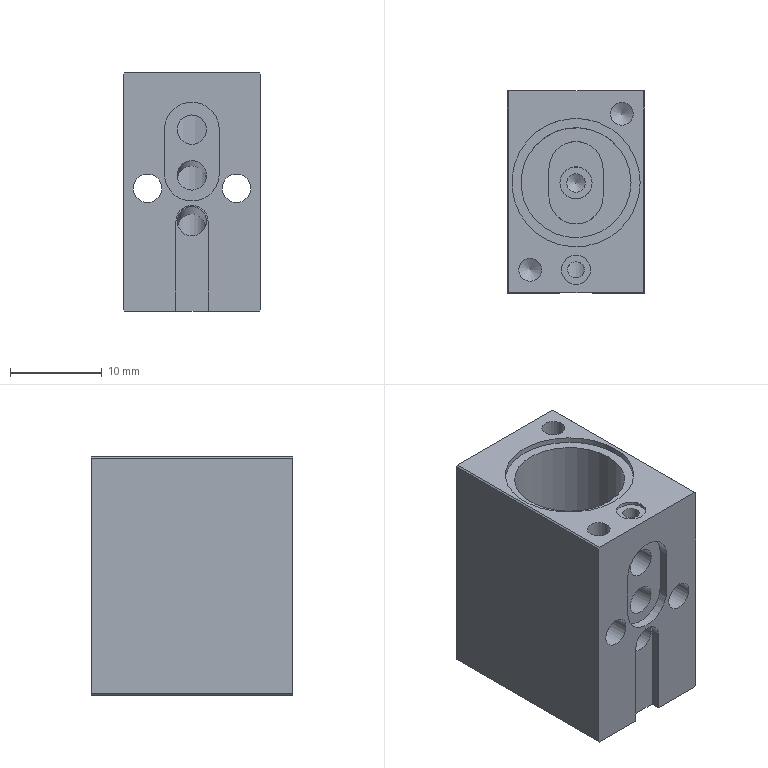Part | 1 solid | 44 faces | box 15 x 22 x 26 mm | volume 6533 mm3 | plane 23 | cylinder 18 | cone 3 | commonest cylinder face diameters 3.2 x4 2.5 x2 3.1 x2 3.5 x2 5.9 x2 6 x2
STEP:
#1=CARTESIAN_POINT('',(-0.01528,-10.,-17.794));
#2=VERTEX_POINT('',#1);
#3=CARTESIAN_POINT('',(-0.01528,-10.,-16.187));
#4=DIRECTION('',(0.,-1.,0.));
#5=DIRECTION('',(0.,0.,-1.));
#6=AXIS2_PLACEMENT_3D('',#3,#4,#5);
#7=ELLIPSE('',#6,1.606,1.6);
#8=EDGE_CURVE('',#2,#2,#7,.T.);
#9=ORIENTED_EDGE('',*,*,#8,.T.);
#10=EDGE_LOOP('',(#9));
#11=FACE_BOUND('',#10,.T.);
#12=CARTESIAN_POINT('',(1.585,0.2576,-17.085));
#13=VERTEX_POINT('',#12);
#14=CARTESIAN_POINT('',(1.488,0.04632,-16.421));
#15=CARTESIAN_POINT('',(1.635,0.3667,-17.087));
#16=CARTESIAN_POINT('',(1.48,0.03243,-17.741));
#17=CARTESIAN_POINT('',(1.041,-0.4993,-18.341));
#18=CARTESIAN_POINT('',(-0.09545,-0.9433,-18.8));
#19=CARTESIAN_POINT('',(-1.156,-0.4116,-18.266));
#20=CARTESIAN_POINT('',(-1.55,0.1565,-17.663));
#21=CARTESIAN_POINT('',(-1.659,0.4306,-16.969));
#22=CARTESIAN_POINT('',(-1.482,0.02854,-16.351));
#23=CARTESIAN_POINT('',(-1.17,-0.3356,-15.874));
#24=CARTESIAN_POINT('',(-0.6683,-0.6615,-15.489));
#25=CARTESIAN_POINT('',(0.02149,-0.7984,-15.334));
#26=CARTESIAN_POINT('',(0.7057,-0.6441,-15.522));
#27=CARTESIAN_POINT('',(1.186,-0.321,-15.926));
#28=CARTESIAN_POINT('',(1.488,0.04632,-16.421));
#29=CARTESIAN_POINT('',(1.635,0.3667,-17.087));
#30=CARTESIAN_POINT('',(1.48,0.03243,-17.741));
#31=B_SPLINE_CURVE_WITH_KNOTS('',3,(#14,#15,#16,#17,#18,#19,#20,#21,#22,#23,#24,#25,#26,#27,#28,#29,#30),.UNSPECIFIED.,.T.,.F.,(1,1,1,1,1,1,1,1,1,1,1,1,1,1,1,1,1,1,1,1,1),(-0.002067,-0.001378,-0.0006891,0.,0.0006891,0.001378,0.002756,0.004134,0.004824,0.005513,0.006202,0.006891,0.00758,0.008269,0.008958,0.009647,0.01034,0.01103,0.01171,0.0124,0.01378),.UNSPECIFIED.);
#32=EDGE_CURVE('',#13,#13,#31,.T.);
#33=ORIENTED_EDGE('',*,*,#32,.T.);
#34=EDGE_LOOP('',(#33));
#35=FACE_BOUND('',#34,.T.);
#36=CARTESIAN_POINT('',(-0.01528,-11.,-16.1));
#37=DIRECTION('',(0.,0.9962,-0.08716));
#38=DIRECTION('',(1.,0.,0.));
#39=AXIS2_PLACEMENT_3D('',#36,#37,#38);
#40=CYLINDRICAL_SURFACE('',#39,1.6);
#41=ADVANCED_FACE('',(#11,#35),#40,.F.);
#42=CARTESIAN_POINT('',(-0.01528,-10.,-12.794));
#43=VERTEX_POINT('',#42);
#44=CARTESIAN_POINT('',(-0.01528,-10.,-11.187));
#45=DIRECTION('',(0.,1.,0.));
#46=DIRECTION('',(0.,0.,-1.));
#47=AXIS2_PLACEMENT_3D('',#44,#45,#46);
#48=ELLIPSE('',#47,1.606,1.6);
#49=EDGE_CURVE('',#43,#43,#48,.T.);
#50=ORIENTED_EDGE('',*,*,#49,.F.);
#51=EDGE_LOOP('',(#50));
#52=FACE_BOUND('',#51,.T.);
#53=CARTESIAN_POINT('',(1.585,-3.038,-11.797));
#54=VERTEX_POINT('',#53);
#55=CARTESIAN_POINT('',(1.252,-3.284,-10.538));
#56=CARTESIAN_POINT('',(1.756,-2.912,-11.798));
#57=CARTESIAN_POINT('',(1.231,-3.297,-13.05));
#58=CARTESIAN_POINT('',(-0.04409,-3.61,-13.528));
#59=CARTESIAN_POINT('',(-1.301,-3.26,-13.012));
#60=CARTESIAN_POINT('',(-1.785,-2.891,-11.745));
#61=CARTESIAN_POINT('',(-1.246,-3.29,-10.505));
#62=CARTESIAN_POINT('',(0.003559,-3.607,-9.965));
#63=CARTESIAN_POINT('',(1.252,-3.284,-10.538));
#64=CARTESIAN_POINT('',(1.756,-2.912,-11.798));
#65=CARTESIAN_POINT('',(1.231,-3.297,-13.05));
#66=B_SPLINE_CURVE_WITH_KNOTS('',3,(#55,#56,#57,#58,#59,#60,#61,#62,#63,#64,#65),.UNSPECIFIED.,.T.,.F.,(1,1,1,1,1,1,1,1,1,1,1,1,1,1,1),(-0.003834,-0.002556,-0.001278,0.,0.001278,0.002556,0.003834,0.005112,0.006391,0.007669,0.008947,0.01022,0.0115,0.01278,0.01406),.UNSPECIFIED.);
#67=EDGE_CURVE('',#54,#54,#66,.T.);
#68=ORIENTED_EDGE('',*,*,#67,.T.);
#69=EDGE_LOOP('',(#68));
#70=FACE_BOUND('',#69,.T.);
#71=CARTESIAN_POINT('',(-0.01528,-11.,-11.1));
#72=DIRECTION('',(0.,0.9962,-0.08716));
#73=DIRECTION('',(1.,0.,0.));
#74=AXIS2_PLACEMENT_3D('',#71,#72,#73);
#75=CYLINDRICAL_SURFACE('',#74,1.6);
#76=ADVANCED_FACE('',(#52,#70),#75,.F.);
#77=CARTESIAN_POINT('',(2.985,-11.,-11.));
#78=VERTEX_POINT('',#77);
#79=CARTESIAN_POINT('',(-3.015,-11.,-11.));
#80=VERTEX_POINT('',#79);
#81=CARTESIAN_POINT('',(-0.01528,-11.,-11.));
#82=DIRECTION('',(0.,1.,0.));
#83=DIRECTION('',(0.,0.,1.));
#84=AXIS2_PLACEMENT_3D('',#81,#82,#83);
#85=CIRCLE('',#84,3.);
#86=EDGE_CURVE('',#78,#80,#85,.T.);
#87=ORIENTED_EDGE('',*,*,#86,.T.);
#88=CARTESIAN_POINT('',(-3.015,-11.,-6.2));
#89=VERTEX_POINT('',#88);
#90=CARTESIAN_POINT('',(-3.015,-11.,-11.));
#91=DIRECTION('',(0.,0.,1.));
#92=VECTOR('',#91,1000.);
#93=LINE('',#90,#92);
#94=EDGE_CURVE('',#80,#89,#93,.T.);
#95=ORIENTED_EDGE('',*,*,#94,.T.);
#96=CARTESIAN_POINT('',(2.985,-11.,-6.2));
#97=VERTEX_POINT('',#96);
#98=CARTESIAN_POINT('',(-0.01528,-11.,-6.2));
#99=DIRECTION('',(0.,1.,0.));
#100=DIRECTION('',(0.,0.,1.));
#101=AXIS2_PLACEMENT_3D('',#98,#99,#100);
#102=CIRCLE('',#101,3.);
#103=EDGE_CURVE('',#89,#97,#102,.T.);
#104=ORIENTED_EDGE('',*,*,#103,.T.);
#105=CARTESIAN_POINT('',(2.985,-11.,-6.2));
#106=DIRECTION('',(0.,0.,-1.));
#107=VECTOR('',#106,1000.);
#108=LINE('',#105,#107);
#109=EDGE_CURVE('',#97,#78,#108,.T.);
#110=ORIENTED_EDGE('',*,*,#109,.T.);
#111=EDGE_LOOP('',(#87,#95,#104,#110));
#112=FACE_BOUND('',#111,.T.);
#113=CARTESIAN_POINT('',(4.85,-11.,-11.05));
#114=VERTEX_POINT('',#113);
#115=CARTESIAN_POINT('',(4.85,-11.,-12.6));
#116=DIRECTION('',(0.,1.,0.));
#117=DIRECTION('',(0.,0.,1.));
#118=AXIS2_PLACEMENT_3D('',#115,#116,#117);
#119=CIRCLE('',#118,1.55);
#120=EDGE_CURVE('',#114,#114,#119,.T.);
#121=ORIENTED_EDGE('',*,*,#120,.T.);
#122=EDGE_LOOP('',(#121));
#123=FACE_BOUND('',#122,.T.);
#124=CARTESIAN_POINT('',(-4.85,-11.,-11.05));
#125=VERTEX_POINT('',#124);
#126=CARTESIAN_POINT('',(-4.85,-11.,-12.6));
#127=DIRECTION('',(0.,1.,0.));
#128=DIRECTION('',(0.,0.,1.));
#129=AXIS2_PLACEMENT_3D('',#126,#127,#128);
#130=CIRCLE('',#129,1.55);
#131=EDGE_CURVE('',#125,#125,#130,.T.);
#132=ORIENTED_EDGE('',*,*,#131,.T.);
#133=EDGE_LOOP('',(#132));
#134=FACE_BOUND('',#133,.T.);
#135=CARTESIAN_POINT('',(-7.5,-11.,-25.85));
#136=VERTEX_POINT('',#135);
#137=CARTESIAN_POINT('',(-7.5,-11.,-0.15));
#138=VERTEX_POINT('',#137);
#139=CARTESIAN_POINT('',(-7.5,-11.,-26.));
#140=DIRECTION('',(0.,0.,1.));
#141=VECTOR('',#140,1000.);
#142=LINE('',#139,#141);
#143=EDGE_CURVE('',#136,#138,#142,.T.);
#144=ORIENTED_EDGE('',*,*,#143,.F.);
#145=CARTESIAN_POINT('',(-7.35,-11.,-26.));
#146=VERTEX_POINT('',#145);
#147=CARTESIAN_POINT('',(-7.35,-11.,-26.));
#148=DIRECTION('',(0.7071,0.,-0.7071));
#149=VECTOR('',#148,1000.);
#150=LINE('',#147,#149);
#151=EDGE_CURVE('',#136,#146,#150,.T.);
#152=ORIENTED_EDGE('',*,*,#151,.T.);
#153=CARTESIAN_POINT('',(-1.75,-11.,-26.));
#154=VERTEX_POINT('',#153);
#155=CARTESIAN_POINT('',(7.5,-11.,-26.));
#156=DIRECTION('',(-1.,0.,0.));
#157=VECTOR('',#156,1000.);
#158=LINE('',#155,#157);
#159=EDGE_CURVE('',#154,#146,#158,.T.);
#160=ORIENTED_EDGE('',*,*,#159,.F.);
#161=CARTESIAN_POINT('',(-1.75,-11.,-16.2));
#162=VERTEX_POINT('',#161);
#163=CARTESIAN_POINT('',(-1.75,-11.,-16.2));
#164=DIRECTION('',(0.,0.,-1.));
#165=VECTOR('',#164,1000.);
#166=LINE('',#163,#165);
#167=EDGE_CURVE('',#162,#154,#166,.T.);
#168=ORIENTED_EDGE('',*,*,#167,.F.);
#169=CARTESIAN_POINT('',(1.75,-11.,-16.2));
#170=VERTEX_POINT('',#169);
#171=CARTESIAN_POINT('',(0.,-11.,-16.2));
#172=DIRECTION('',(0.,-1.,0.));
#173=DIRECTION('',(0.,0.,1.));
#174=AXIS2_PLACEMENT_3D('',#171,#172,#173);
#175=CIRCLE('',#174,1.75);
#176=EDGE_CURVE('',#170,#162,#175,.T.);
#177=ORIENTED_EDGE('',*,*,#176,.F.);
#178=CARTESIAN_POINT('',(1.75,-11.,-26.));
#179=VERTEX_POINT('',#178);
#180=CARTESIAN_POINT('',(1.75,-11.,-26.));
#181=DIRECTION('',(0.,0.,1.));
#182=VECTOR('',#181,1000.);
#183=LINE('',#180,#182);
#184=EDGE_CURVE('',#179,#170,#183,.T.);
#185=ORIENTED_EDGE('',*,*,#184,.F.);
#186=CARTESIAN_POINT('',(7.35,-11.,-26.));
#187=VERTEX_POINT('',#186);
#188=CARTESIAN_POINT('',(7.5,-11.,-26.));
#189=DIRECTION('',(-1.,0.,0.));
#190=VECTOR('',#189,1000.);
#191=LINE('',#188,#190);
#192=EDGE_CURVE('',#187,#179,#191,.T.);
#193=ORIENTED_EDGE('',*,*,#192,.F.);
#194=CARTESIAN_POINT('',(7.5,-11.,-25.85));
#195=VERTEX_POINT('',#194);
#196=CARTESIAN_POINT('',(7.35,-11.,-26.));
#197=DIRECTION('',(0.7071,0.,0.7071));
#198=VECTOR('',#197,1000.);
#199=LINE('',#196,#198);
#200=EDGE_CURVE('',#187,#195,#199,.T.);
#201=ORIENTED_EDGE('',*,*,#200,.T.);
#202=CARTESIAN_POINT('',(7.5,-11.,-0.15));
#203=VERTEX_POINT('',#202);
#204=CARTESIAN_POINT('',(7.5,-11.,-26.));
#205=DIRECTION('',(0.,0.,1.));
#206=VECTOR('',#205,1000.);
#207=LINE('',#204,#206);
#208=EDGE_CURVE('',#195,#203,#207,.T.);
#209=ORIENTED_EDGE('',*,*,#208,.T.);
#210=CARTESIAN_POINT('',(7.35,-11.,0.));
#211=VERTEX_POINT('',#210);
#212=CARTESIAN_POINT('',(7.5,-11.,-0.15));
#213=DIRECTION('',(0.7071,0.,-0.7071));
#214=VECTOR('',#213,1000.);
#215=LINE('',#212,#214);
#216=EDGE_CURVE('',#203,#211,#215,.F.);
#217=ORIENTED_EDGE('',*,*,#216,.T.);
#218=CARTESIAN_POINT('',(-7.35,-11.,0.));
#219=VERTEX_POINT('',#218);
#220=CARTESIAN_POINT('',(7.5,-11.,0.));
#221=DIRECTION('',(-1.,0.,0.));
#222=VECTOR('',#221,1000.);
#223=LINE('',#220,#222);
#224=EDGE_CURVE('',#211,#219,#223,.T.);
#225=ORIENTED_EDGE('',*,*,#224,.T.);
#226=CARTESIAN_POINT('',(-7.5,-11.,-0.15));
#227=DIRECTION('',(0.7071,0.,0.7071));
#228=VECTOR('',#227,1000.);
#229=LINE('',#226,#228);
#230=EDGE_CURVE('',#219,#138,#229,.F.);
#231=ORIENTED_EDGE('',*,*,#230,.T.);
#232=EDGE_LOOP('',(#144,#152,#160,#168,#177,#185,#193,#201,#209,#217,#225,#231));
#233=FACE_BOUND('',#232,.T.);
#234=CARTESIAN_POINT('',(7.5,-11.,-26.));
#235=DIRECTION('',(0.,1.,0.));
#236=DIRECTION('',(0.,0.,1.));
#237=AXIS2_PLACEMENT_3D('',#234,#235,#236);
#238=PLANE('',#237);
#239=ADVANCED_FACE('',(#112,#123,#134,#233),#238,.F.);
#240=ORIENTED_EDGE('',*,*,#159,.T.);
#241=CARTESIAN_POINT('',(-7.35,11.,-26.));
#242=VERTEX_POINT('',#241);
#243=CARTESIAN_POINT('',(-7.35,11.,-26.));
#244=DIRECTION('',(0.,1.,0.));
#245=VECTOR('',#244,1000.);
#246=LINE('',#243,#245);
#247=EDGE_CURVE('',#146,#242,#246,.T.);
#248=ORIENTED_EDGE('',*,*,#247,.T.);
#249=CARTESIAN_POINT('',(7.35,11.,-26.));
#250=VERTEX_POINT('',#249);
#251=CARTESIAN_POINT('',(-7.5,11.,-26.));
#252=DIRECTION('',(1.,0.,0.));
#253=VECTOR('',#252,1000.);
#254=LINE('',#251,#253);
#255=EDGE_CURVE('',#242,#250,#254,.T.);
#256=ORIENTED_EDGE('',*,*,#255,.T.);
#257=CARTESIAN_POINT('',(7.35,-11.,-26.));
#258=DIRECTION('',(0.,-1.,0.));
#259=VECTOR('',#258,1000.);
#260=LINE('',#257,#259);
#261=EDGE_CURVE('',#250,#187,#260,.T.);
#262=ORIENTED_EDGE('',*,*,#261,.T.);
#263=ORIENTED_EDGE('',*,*,#192,.T.);
#264=CARTESIAN_POINT('',(1.75,-10.,-26.));
#265=VERTEX_POINT('',#264);
#266=CARTESIAN_POINT('',(1.75,-10.,-26.));
#267=DIRECTION('',(0.,-1.,0.));
#268=VECTOR('',#267,1000.);
#269=LINE('',#266,#268);
#270=EDGE_CURVE('',#265,#179,#269,.T.);
#271=ORIENTED_EDGE('',*,*,#270,.F.);
#272=CARTESIAN_POINT('',(-1.75,-10.,-26.));
#273=VERTEX_POINT('',#272);
#274=CARTESIAN_POINT('',(-1.75,-10.,-26.));
#275=DIRECTION('',(1.,0.,0.));
#276=VECTOR('',#275,1000.);
#277=LINE('',#274,#276);
#278=EDGE_CURVE('',#273,#265,#277,.T.);
#279=ORIENTED_EDGE('',*,*,#278,.F.);
#280=CARTESIAN_POINT('',(-1.75,-10.,-26.));
#281=DIRECTION('',(0.,-1.,0.));
#282=VECTOR('',#281,1000.);
#283=LINE('',#280,#282);
#284=EDGE_CURVE('',#273,#154,#283,.T.);
#285=ORIENTED_EDGE('',*,*,#284,.T.);
#286=EDGE_LOOP('',(#240,#248,#256,#262,#263,#271,#279,#285));
#287=FACE_BOUND('',#286,.T.);
#288=CARTESIAN_POINT('',(0.,0.,-26.));
#289=DIRECTION('',(0.,0.,-1.));
#290=DIRECTION('',(-1.,0.,0.));
#291=AXIS2_PLACEMENT_3D('',#288,#289,#290);
#292=PLANE('',#291);
#293=ADVANCED_FACE('',(#287),#292,.T.);
#294=ORIENTED_EDGE('',*,*,#131,.F.);
#295=EDGE_LOOP('',(#294));
#296=FACE_BOUND('',#295,.T.);
#297=CARTESIAN_POINT('',(-4.85,11.,-14.15));
#298=VERTEX_POINT('',#297);
#299=CARTESIAN_POINT('',(-4.85,11.,-12.6));
#300=DIRECTION('',(0.,-1.,0.));
#301=DIRECTION('',(0.,0.,-1.));
#302=AXIS2_PLACEMENT_3D('',#299,#300,#301);
#303=CIRCLE('',#302,1.55);
#304=EDGE_CURVE('',#298,#298,#303,.F.);
#305=ORIENTED_EDGE('',*,*,#304,.T.);
#306=EDGE_LOOP('',(#305));
#307=FACE_BOUND('',#306,.T.);
#308=CARTESIAN_POINT('',(-4.85,-11.,-12.6));
#309=DIRECTION('',(0.,1.,0.));
#310=DIRECTION('',(1.,0.,0.));
#311=AXIS2_PLACEMENT_3D('',#308,#309,#310);
#312=CYLINDRICAL_SURFACE('',#311,1.55);
#313=ADVANCED_FACE('',(#296,#307),#312,.F.);
#314=CARTESIAN_POINT('',(-7.5,11.,-25.85));
#315=VERTEX_POINT('',#314);
#316=CARTESIAN_POINT('',(-7.5,11.,-0.15));
#317=VERTEX_POINT('',#316);
#318=CARTESIAN_POINT('',(-7.5,11.,-26.));
#319=DIRECTION('',(0.,0.,1.));
#320=VECTOR('',#319,1000.);
#321=LINE('',#318,#320);
#322=EDGE_CURVE('',#315,#317,#321,.T.);
#323=ORIENTED_EDGE('',*,*,#322,.F.);
#324=CARTESIAN_POINT('',(-7.5,-11.,-25.85));
#325=DIRECTION('',(0.,-1.,0.));
#326=VECTOR('',#325,1000.);
#327=LINE('',#324,#326);
#328=EDGE_CURVE('',#315,#136,#327,.T.);
#329=ORIENTED_EDGE('',*,*,#328,.T.);
#330=ORIENTED_EDGE('',*,*,#143,.T.);
#331=CARTESIAN_POINT('',(-7.5,-11.,-0.15));
#332=DIRECTION('',(0.,1.,0.));
#333=VECTOR('',#332,1000.);
#334=LINE('',#331,#333);
#335=EDGE_CURVE('',#138,#317,#334,.T.);
#336=ORIENTED_EDGE('',*,*,#335,.T.);
#337=EDGE_LOOP('',(#323,#329,#330,#336));
#338=FACE_BOUND('',#337,.T.);
#339=CARTESIAN_POINT('',(-7.5,-11.,-26.));
#340=DIRECTION('',(1.,0.,0.));
#341=DIRECTION('',(0.,0.,-1.));
#342=AXIS2_PLACEMENT_3D('',#339,#340,#341);
#343=PLANE('',#342);
#344=ADVANCED_FACE('',(#338),#343,.F.);
#345=ORIENTED_EDGE('',*,*,#304,.F.);
#346=EDGE_LOOP('',(#345));
#347=FACE_BOUND('',#346,.T.);
#348=CARTESIAN_POINT('',(4.85,11.,-14.15));
#349=VERTEX_POINT('',#348);
#350=CARTESIAN_POINT('',(4.85,11.,-12.6));
#351=DIRECTION('',(0.,-1.,0.));
#352=DIRECTION('',(0.,0.,-1.));
#353=AXIS2_PLACEMENT_3D('',#350,#351,#352);
#354=CIRCLE('',#353,1.55);
#355=EDGE_CURVE('',#349,#349,#354,.T.);
#356=ORIENTED_EDGE('',*,*,#355,.T.);
#357=EDGE_LOOP('',(#356));
#358=FACE_BOUND('',#357,.T.);
#359=ORIENTED_EDGE('',*,*,#255,.F.);
#360=CARTESIAN_POINT('',(-7.35,11.,-26.));
#361=DIRECTION('',(-0.7071,0.,0.7071));
#362=VECTOR('',#361,1000.);
#363=LINE('',#360,#362);
#364=EDGE_CURVE('',#242,#315,#363,.T.);
#365=ORIENTED_EDGE('',*,*,#364,.T.);
#366=ORIENTED_EDGE('',*,*,#322,.T.);
#367=CARTESIAN_POINT('',(-7.35,11.,0.));
#368=VERTEX_POINT('',#367);
#369=CARTESIAN_POINT('',(-7.5,11.,-0.15));
#370=DIRECTION('',(-0.7071,0.,-0.7071));
#371=VECTOR('',#370,1000.);
#372=LINE('',#369,#371);
#373=EDGE_CURVE('',#317,#368,#372,.F.);
#374=ORIENTED_EDGE('',*,*,#373,.T.);
#375=CARTESIAN_POINT('',(7.35,11.,0.));
#376=VERTEX_POINT('',#375);
#377=CARTESIAN_POINT('',(-7.5,11.,0.));
#378=DIRECTION('',(1.,0.,0.));
#379=VECTOR('',#378,1000.);
#380=LINE('',#377,#379);
#381=EDGE_CURVE('',#368,#376,#380,.T.);
#382=ORIENTED_EDGE('',*,*,#381,.T.);
#383=CARTESIAN_POINT('',(7.5,11.,-0.15));
#384=VERTEX_POINT('',#383);
#385=CARTESIAN_POINT('',(7.5,11.,-0.15));
#386=DIRECTION('',(-0.7071,0.,0.7071));
#387=VECTOR('',#386,1000.);
#388=LINE('',#385,#387);
#389=EDGE_CURVE('',#376,#384,#388,.F.);
#390=ORIENTED_EDGE('',*,*,#389,.T.);
#391=CARTESIAN_POINT('',(7.5,11.,-25.85));
#392=VERTEX_POINT('',#391);
#393=CARTESIAN_POINT('',(7.5,11.,-26.));
#394=DIRECTION('',(0.,0.,1.));
#395=VECTOR('',#394,1000.);
#396=LINE('',#393,#395);
#397=EDGE_CURVE('',#392,#384,#396,.T.);
#398=ORIENTED_EDGE('',*,*,#397,.F.);
#399=CARTESIAN_POINT('',(7.35,11.,-26.));
#400=DIRECTION('',(-0.7071,0.,-0.7071));
#401=VECTOR('',#400,1000.);
#402=LINE('',#399,#401);
#403=EDGE_CURVE('',#392,#250,#402,.T.);
#404=ORIENTED_EDGE('',*,*,#403,.T.);
#405=EDGE_LOOP('',(#359,#365,#366,#374,#382,#390,#398,#404));
#406=FACE_BOUND('',#405,.T.);
#407=CARTESIAN_POINT('',(-7.5,11.,-26.));
#408=DIRECTION('',(0.,-1.,0.));
#409=DIRECTION('',(0.,0.,-1.));
#410=AXIS2_PLACEMENT_3D('',#407,#408,#409);
#411=PLANE('',#410);
#412=ADVANCED_FACE('',(#347,#358,#406),#411,.F.);
#413=ORIENTED_EDGE('',*,*,#208,.F.);
#414=CARTESIAN_POINT('',(7.5,11.,-25.85));
#415=DIRECTION('',(0.,1.,0.));
#416=VECTOR('',#415,1000.);
#417=LINE('',#414,#416);
#418=EDGE_CURVE('',#195,#392,#417,.T.);
#419=ORIENTED_EDGE('',*,*,#418,.T.);
#420=ORIENTED_EDGE('',*,*,#397,.T.);
#421=CARTESIAN_POINT('',(7.5,11.,-0.15));
#422=DIRECTION('',(0.,-1.,0.));
#423=VECTOR('',#422,1000.);
#424=LINE('',#421,#423);
#425=EDGE_CURVE('',#384,#203,#424,.T.);
#426=ORIENTED_EDGE('',*,*,#425,.T.);
#427=EDGE_LOOP('',(#413,#419,#420,#426));
#428=FACE_BOUND('',#427,.T.);
#429=CARTESIAN_POINT('',(7.5,11.,-26.));
#430=DIRECTION('',(-1.,0.,0.));
#431=DIRECTION('',(0.,0.,1.));
#432=AXIS2_PLACEMENT_3D('',#429,#430,#431);
#433=PLANE('',#432);
#434=ADVANCED_FACE('',(#428),#433,.F.);
#435=CARTESIAN_POINT('',(1.6,-8.5,0.));
#436=VERTEX_POINT('',#435);
#437=CARTESIAN_POINT('',(0.,-8.5,0.));
#438=DIRECTION('',(0.,0.,1.));
#439=DIRECTION('',(1.,0.,0.));
#440=AXIS2_PLACEMENT_3D('',#437,#438,#439);
#441=CIRCLE('',#440,1.6);
#442=EDGE_CURVE('',#436,#436,#441,.T.);
#443=ORIENTED_EDGE('',*,*,#442,.F.);
#444=EDGE_LOOP('',(#443));
#445=FACE_BOUND('',#444,.T.);
#446=CARTESIAN_POINT('',(-6.25,-8.5,0.));
#447=VERTEX_POINT('',#446);
#448=CARTESIAN_POINT('',(-5.,-8.5,0.));
#449=DIRECTION('',(0.,0.,-1.));
#450=DIRECTION('',(-1.,0.,0.));
#451=AXIS2_PLACEMENT_3D('',#448,#449,#450);
#452=CIRCLE('',#451,1.25);
#453=EDGE_CURVE('',#447,#447,#452,.T.);
#454=ORIENTED_EDGE('',*,*,#453,.T.);
#455=EDGE_LOOP('',(#454));
#456=FACE_BOUND('',#455,.T.);
#457=CARTESIAN_POINT('',(3.75,8.5,0.));
#458=VERTEX_POINT('',#457);
#459=CARTESIAN_POINT('',(5.,8.5,0.));
#460=DIRECTION('',(0.,0.,-1.));
#461=DIRECTION('',(-1.,0.,0.));
#462=AXIS2_PLACEMENT_3D('',#459,#460,#461);
#463=CIRCLE('',#462,1.25);
#464=EDGE_CURVE('',#458,#458,#463,.T.);
#465=ORIENTED_EDGE('',*,*,#464,.T.);
#466=EDGE_LOOP('',(#465));
#467=FACE_BOUND('',#466,.T.);
#468=CARTESIAN_POINT('',(7.,1.,0.));
#469=VERTEX_POINT('',#468);
#470=CARTESIAN_POINT('',(0.,1.,0.));
#471=DIRECTION('',(0.,0.,1.));
#472=DIRECTION('',(1.,0.,0.));
#473=AXIS2_PLACEMENT_3D('',#470,#471,#472);
#474=CIRCLE('',#473,7.);
#475=EDGE_CURVE('',#469,#469,#474,.T.);
#476=ORIENTED_EDGE('',*,*,#475,.F.);
#477=EDGE_LOOP('',(#476));
#478=FACE_BOUND('',#477,.T.);
#479=ORIENTED_EDGE('',*,*,#224,.F.);
#480=CARTESIAN_POINT('',(7.35,0.,0.));
#481=DIRECTION('',(0.,1.,0.));
#482=VECTOR('',#481,1000.);
#483=LINE('',#480,#482);
#484=EDGE_CURVE('',#211,#376,#483,.T.);
#485=ORIENTED_EDGE('',*,*,#484,.T.);
#486=ORIENTED_EDGE('',*,*,#381,.F.);
#487=CARTESIAN_POINT('',(-7.35,0.,0.));
#488=DIRECTION('',(0.,-1.,0.));
#489=VECTOR('',#488,1000.);
#490=LINE('',#487,#489);
#491=EDGE_CURVE('',#368,#219,#490,.T.);
#492=ORIENTED_EDGE('',*,*,#491,.T.);
#493=EDGE_LOOP('',(#479,#485,#486,#492));
#494=FACE_BOUND('',#493,.T.);
#495=CARTESIAN_POINT('',(0.,0.,0.));
#496=DIRECTION('',(0.,0.,-1.));
#497=DIRECTION('',(-1.,0.,0.));
#498=AXIS2_PLACEMENT_3D('',#495,#496,#497);
#499=PLANE('',#498);
#500=ADVANCED_FACE('',(#445,#456,#467,#478,#494),#499,.F.);
#501=CARTESIAN_POINT('',(7.,1.,-0.6));
#502=VERTEX_POINT('',#501);
#503=CARTESIAN_POINT('',(0.,1.,-0.6));
#504=DIRECTION('',(0.,0.,1.));
#505=DIRECTION('',(1.,0.,0.));
#506=AXIS2_PLACEMENT_3D('',#503,#504,#505);
#507=CIRCLE('',#506,7.);
#508=EDGE_CURVE('',#502,#502,#507,.F.);
#509=ORIENTED_EDGE('',*,*,#508,.T.);
#510=EDGE_LOOP('',(#509));
#511=FACE_BOUND('',#510,.T.);
#512=ORIENTED_EDGE('',*,*,#475,.T.);
#513=EDGE_LOOP('',(#512));
#514=FACE_BOUND('',#513,.T.);
#515=CARTESIAN_POINT('',(0.,1.,-0.6));
#516=DIRECTION('',(0.,0.,1.));
#517=DIRECTION('',(1.,0.,0.));
#518=AXIS2_PLACEMENT_3D('',#515,#516,#517);
#519=CYLINDRICAL_SURFACE('',#518,7.);
#520=ADVANCED_FACE('',(#511,#514),#519,.F.);
#521=CARTESIAN_POINT('',(6.,1.,-0.6));
#522=VERTEX_POINT('',#521);
#523=CARTESIAN_POINT('',(0.,1.,-0.6));
#524=DIRECTION('',(0.,0.,1.));
#525=DIRECTION('',(1.,0.,0.));
#526=AXIS2_PLACEMENT_3D('',#523,#524,#525);
#527=CIRCLE('',#526,6.);
#528=EDGE_CURVE('',#522,#522,#527,.T.);
#529=ORIENTED_EDGE('',*,*,#528,.F.);
#530=EDGE_LOOP('',(#529));
#531=FACE_BOUND('',#530,.T.);
#532=ORIENTED_EDGE('',*,*,#508,.F.);
#533=EDGE_LOOP('',(#532));
#534=FACE_BOUND('',#533,.T.);
#535=CARTESIAN_POINT('',(0.,1.,-0.6));
#536=DIRECTION('',(0.,0.,1.));
#537=DIRECTION('',(1.,0.,0.));
#538=AXIS2_PLACEMENT_3D('',#535,#536,#537);
#539=PLANE('',#538);
#540=ADVANCED_FACE('',(#531,#534),#539,.T.);
#541=CARTESIAN_POINT('',(-0.01528,-5.,-4.6));
#542=VERTEX_POINT('',#541);
#543=CARTESIAN_POINT('',(1.24,-4.896,-4.947));
#544=CARTESIAN_POINT('',(-0.01563,-5.053,-4.426));
#545=CARTESIAN_POINT('',(-1.269,-4.89,-4.947));
#546=CARTESIAN_POINT('',(-1.788,-4.723,-6.198));
#547=CARTESIAN_POINT('',(-1.269,-4.89,-7.454));
#548=CARTESIAN_POINT('',(-0.01711,-5.053,-7.973));
#549=CARTESIAN_POINT('',(1.237,-4.897,-7.455));
#550=CARTESIAN_POINT('',(1.758,-4.732,-6.201));
#551=CARTESIAN_POINT('',(1.24,-4.896,-4.947));
#552=CARTESIAN_POINT('',(-0.01563,-5.053,-4.426));
#553=CARTESIAN_POINT('',(-1.269,-4.89,-4.947));
#554=B_SPLINE_CURVE_WITH_KNOTS('',3,(#543,#544,#545,#546,#547,#548,#549,#550,#551,#552,#553),.UNSPECIFIED.,.T.,.F.,(1,1,1,1,1,1,1,1,1,1,1,1,1,1,1),(-0.003768,-0.002512,-0.001256,0.,0.001256,0.002512,0.003768,0.005024,0.006281,0.007537,0.008793,0.01005,0.01131,0.01256,0.01382),.UNSPECIFIED.);
#555=EDGE_CURVE('',#542,#542,#554,.T.);
#556=ORIENTED_EDGE('',*,*,#555,.T.);
#557=EDGE_LOOP('',(#556));
#558=FACE_BOUND('',#557,.T.);
#559=ORIENTED_EDGE('',*,*,#528,.T.);
#560=EDGE_LOOP('',(#559));
#561=FACE_BOUND('',#560,.T.);
#562=CARTESIAN_POINT('',(6.,1.,-9.2));
#563=VERTEX_POINT('',#562);
#564=CARTESIAN_POINT('',(0.,1.,-9.2));
#565=DIRECTION('',(0.,0.,1.));
#566=DIRECTION('',(1.,0.,0.));
#567=AXIS2_PLACEMENT_3D('',#564,#565,#566);
#568=CIRCLE('',#567,6.);
#569=EDGE_CURVE('',#563,#563,#568,.F.);
#570=ORIENTED_EDGE('',*,*,#569,.T.);
#571=EDGE_LOOP('',(#570));
#572=FACE_BOUND('',#571,.T.);
#573=CARTESIAN_POINT('',(0.,1.,-9.2));
#574=DIRECTION('',(0.,0.,1.));
#575=DIRECTION('',(1.,0.,0.));
#576=AXIS2_PLACEMENT_3D('',#573,#574,#575);
#577=CYLINDRICAL_SURFACE('',#576,6.);
#578=ADVANCED_FACE('',(#558,#561,#572),#577,.F.);
#579=CARTESIAN_POINT('',(2.95,2.55,-9.2));
#580=VERTEX_POINT('',#579);
#581=CARTESIAN_POINT('',(-2.95,2.55,-9.2));
#582=VERTEX_POINT('',#581);
#583=CARTESIAN_POINT('',(0.,2.55,-9.2));
#584=DIRECTION('',(0.,0.,1.));
#585=DIRECTION('',(1.,0.,0.));
#586=AXIS2_PLACEMENT_3D('',#583,#584,#585);
#587=CIRCLE('',#586,2.95);
#588=EDGE_CURVE('',#580,#582,#587,.T.);
#589=ORIENTED_EDGE('',*,*,#588,.F.);
#590=CARTESIAN_POINT('',(2.95,-0.55,-9.2));
#591=VERTEX_POINT('',#590);
#592=CARTESIAN_POINT('',(2.95,1.,-9.2));
#593=DIRECTION('',(0.,1.,0.));
#594=VECTOR('',#593,1000.);
#595=LINE('',#592,#594);
#596=EDGE_CURVE('',#591,#580,#595,.T.);
#597=ORIENTED_EDGE('',*,*,#596,.F.);
#598=CARTESIAN_POINT('',(-2.95,-0.55,-9.2));
#599=VERTEX_POINT('',#598);
#600=CARTESIAN_POINT('',(0.,-0.55,-9.2));
#601=DIRECTION('',(0.,0.,1.));
#602=DIRECTION('',(1.,0.,0.));
#603=AXIS2_PLACEMENT_3D('',#600,#601,#602);
#604=CIRCLE('',#603,2.95);
#605=EDGE_CURVE('',#599,#591,#604,.T.);
#606=ORIENTED_EDGE('',*,*,#605,.F.);
#607=CARTESIAN_POINT('',(-2.95,1.,-9.2));
#608=DIRECTION('',(0.,-1.,0.));
#609=VECTOR('',#608,1000.);
#610=LINE('',#607,#609);
#611=EDGE_CURVE('',#582,#599,#610,.T.);
#612=ORIENTED_EDGE('',*,*,#611,.F.);
#613=EDGE_LOOP('',(#589,#597,#606,#612));
#614=FACE_BOUND('',#613,.T.);
#615=ORIENTED_EDGE('',*,*,#569,.F.);
#616=EDGE_LOOP('',(#615));
#617=FACE_BOUND('',#616,.T.);
#618=CARTESIAN_POINT('',(0.,1.,-9.2));
#619=DIRECTION('',(0.,0.,1.));
#620=DIRECTION('',(1.,0.,0.));
#621=AXIS2_PLACEMENT_3D('',#618,#619,#620);
#622=PLANE('',#621);
#623=ADVANCED_FACE('',(#614,#617),#622,.T.);
#624=ORIENTED_EDGE('',*,*,#588,.T.);
#625=CARTESIAN_POINT('',(-2.95,2.55,-13.7));
#626=VERTEX_POINT('',#625);
#627=CARTESIAN_POINT('',(-2.95,2.55,-13.8));
#628=DIRECTION('',(0.,0.,1.));
#629=VECTOR('',#628,1000.);
#630=LINE('',#627,#629);
#631=EDGE_CURVE('',#582,#626,#630,.F.);
#632=ORIENTED_EDGE('',*,*,#631,.T.);
#633=CARTESIAN_POINT('',(2.95,2.55,-13.7));
#634=VERTEX_POINT('',#633);
#635=CARTESIAN_POINT('',(0.,2.55,-13.7));
#636=DIRECTION('',(0.,0.,1.));
#637=DIRECTION('',(1.,0.,0.));
#638=AXIS2_PLACEMENT_3D('',#635,#636,#637);
#639=CIRCLE('',#638,2.95);
#640=EDGE_CURVE('',#626,#634,#639,.F.);
#641=ORIENTED_EDGE('',*,*,#640,.T.);
#642=CARTESIAN_POINT('',(2.95,2.55,-13.8));
#643=DIRECTION('',(0.,0.,1.));
#644=VECTOR('',#643,1000.);
#645=LINE('',#642,#644);
#646=EDGE_CURVE('',#580,#634,#645,.F.);
#647=ORIENTED_EDGE('',*,*,#646,.F.);
#648=EDGE_LOOP('',(#624,#632,#641,#647));
#649=FACE_BOUND('',#648,.T.);
#650=CARTESIAN_POINT('',(0.,2.55,-13.8));
#651=DIRECTION('',(0.,0.,1.));
#652=DIRECTION('',(1.,0.,0.));
#653=AXIS2_PLACEMENT_3D('',#650,#651,#652);
#654=CYLINDRICAL_SURFACE('',#653,2.95);
#655=ADVANCED_FACE('',(#649),#654,.F.);
#656=ORIENTED_EDGE('',*,*,#611,.T.);
#657=CARTESIAN_POINT('',(-2.95,-0.55,-13.7));
#658=VERTEX_POINT('',#657);
#659=CARTESIAN_POINT('',(-2.95,-0.55,-13.8));
#660=DIRECTION('',(0.,0.,1.));
#661=VECTOR('',#660,1000.);
#662=LINE('',#659,#661);
#663=EDGE_CURVE('',#599,#658,#662,.F.);
#664=ORIENTED_EDGE('',*,*,#663,.T.);
#665=CARTESIAN_POINT('',(-2.95,2.4,-13.7));
#666=DIRECTION('',(0.,1.,0.));
#667=VECTOR('',#666,1000.);
#668=LINE('',#665,#667);
#669=EDGE_CURVE('',#658,#626,#668,.T.);
#670=ORIENTED_EDGE('',*,*,#669,.T.);
#671=ORIENTED_EDGE('',*,*,#631,.F.);
#672=EDGE_LOOP('',(#656,#664,#670,#671));
#673=FACE_BOUND('',#672,.T.);
#674=CARTESIAN_POINT('',(-2.95,2.4,-13.8));
#675=DIRECTION('',(-1.,0.,0.));
#676=DIRECTION('',(0.,-1.,0.));
#677=AXIS2_PLACEMENT_3D('',#674,#675,#676);
#678=PLANE('',#677);
#679=ADVANCED_FACE('',(#673),#678,.F.);
#680=ORIENTED_EDGE('',*,*,#67,.F.);
#681=EDGE_LOOP('',(#680));
#682=FACE_BOUND('',#681,.T.);
#683=ORIENTED_EDGE('',*,*,#605,.T.);
#684=CARTESIAN_POINT('',(2.95,-0.55,-13.7));
#685=VERTEX_POINT('',#684);
#686=CARTESIAN_POINT('',(2.95,-0.55,-13.8));
#687=DIRECTION('',(0.,0.,1.));
#688=VECTOR('',#687,1000.);
#689=LINE('',#686,#688);
#690=EDGE_CURVE('',#591,#685,#689,.F.);
#691=ORIENTED_EDGE('',*,*,#690,.T.);
#692=CARTESIAN_POINT('',(0.,-0.55,-13.7));
#693=DIRECTION('',(0.,0.,1.));
#694=DIRECTION('',(1.,0.,0.));
#695=AXIS2_PLACEMENT_3D('',#692,#693,#694);
#696=CIRCLE('',#695,2.95);
#697=EDGE_CURVE('',#685,#658,#696,.F.);
#698=ORIENTED_EDGE('',*,*,#697,.T.);
#699=ORIENTED_EDGE('',*,*,#663,.F.);
#700=EDGE_LOOP('',(#683,#691,#698,#699));
#701=FACE_BOUND('',#700,.T.);
#702=CARTESIAN_POINT('',(0.,-0.55,-13.8));
#703=DIRECTION('',(0.,0.,1.));
#704=DIRECTION('',(1.,0.,0.));
#705=AXIS2_PLACEMENT_3D('',#702,#703,#704);
#706=CYLINDRICAL_SURFACE('',#705,2.95);
#707=ADVANCED_FACE('',(#682,#701),#706,.F.);
#708=ORIENTED_EDGE('',*,*,#596,.T.);
#709=ORIENTED_EDGE('',*,*,#646,.T.);
#710=CARTESIAN_POINT('',(2.95,-0.4,-13.7));
#711=DIRECTION('',(0.,-1.,0.));
#712=VECTOR('',#711,1000.);
#713=LINE('',#710,#712);
#714=EDGE_CURVE('',#634,#685,#713,.T.);
#715=ORIENTED_EDGE('',*,*,#714,.T.);
#716=ORIENTED_EDGE('',*,*,#690,.F.);
#717=EDGE_LOOP('',(#708,#709,#715,#716));
#718=FACE_BOUND('',#717,.T.);
#719=CARTESIAN_POINT('',(2.95,-0.4,-13.8));
#720=DIRECTION('',(1.,0.,0.));
#721=DIRECTION('',(0.,0.,-1.));
#722=AXIS2_PLACEMENT_3D('',#719,#720,#721);
#723=PLANE('',#722);
#724=ADVANCED_FACE('',(#718),#723,.F.);
#725=CARTESIAN_POINT('',(1.75,1.,-13.7));
#726=VERTEX_POINT('',#725);
#727=CARTESIAN_POINT('',(0.,1.,-13.7));
#728=DIRECTION('',(0.,0.,1.));
#729=DIRECTION('',(1.,0.,0.));
#730=AXIS2_PLACEMENT_3D('',#727,#728,#729);
#731=CIRCLE('',#730,1.75);
#732=EDGE_CURVE('',#726,#726,#731,.T.);
#733=ORIENTED_EDGE('',*,*,#732,.F.);
#734=EDGE_LOOP('',(#733));
#735=FACE_BOUND('',#734,.T.);
#736=ORIENTED_EDGE('',*,*,#640,.F.);
#737=ORIENTED_EDGE('',*,*,#669,.F.);
#738=ORIENTED_EDGE('',*,*,#697,.F.);
#739=ORIENTED_EDGE('',*,*,#714,.F.);
#740=EDGE_LOOP('',(#736,#737,#738,#739));
#741=FACE_BOUND('',#740,.T.);
#742=CARTESIAN_POINT('',(0.,2.4,-13.7));
#743=DIRECTION('',(0.,0.,1.));
#744=DIRECTION('',(1.,0.,0.));
#745=AXIS2_PLACEMENT_3D('',#742,#743,#744);
#746=PLANE('',#745);
#747=ADVANCED_FACE('',(#735,#741),#746,.T.);
#748=CARTESIAN_POINT('',(-1.,1.,-21.1));
#749=VERTEX_POINT('',#748);
#750=CARTESIAN_POINT('',(0.,1.,-21.1));
#751=DIRECTION('',(0.,0.,-1.));
#752=DIRECTION('',(-1.,0.,0.));
#753=AXIS2_PLACEMENT_3D('',#750,#751,#752);
#754=CIRCLE('',#753,1.);
#755=EDGE_CURVE('',#749,#749,#754,.T.);
#756=ORIENTED_EDGE('',*,*,#755,.T.);
#757=EDGE_LOOP('',(#756));
#758=FACE_BOUND('',#757,.T.);
#759=CARTESIAN_POINT('',(-1.75,1.,-21.1));
#760=VERTEX_POINT('',#759);
#761=CARTESIAN_POINT('',(0.,1.,-21.1));
#762=DIRECTION('',(0.,0.,-1.));
#763=DIRECTION('',(-1.,0.,0.));
#764=AXIS2_PLACEMENT_3D('',#761,#762,#763);
#765=CIRCLE('',#764,1.75);
#766=EDGE_CURVE('',#760,#760,#765,.T.);
#767=ORIENTED_EDGE('',*,*,#766,.F.);
#768=EDGE_LOOP('',(#767));
#769=FACE_BOUND('',#768,.T.);
#770=CARTESIAN_POINT('',(0.,1.,-21.1));
#771=DIRECTION('',(0.,0.,-1.));
#772=DIRECTION('',(-1.,0.,0.));
#773=AXIS2_PLACEMENT_3D('',#770,#771,#772);
#774=PLANE('',#773);
#775=ADVANCED_FACE('',(#758,#769),#774,.F.);
#776=ORIENTED_EDGE('',*,*,#32,.F.);
#777=EDGE_LOOP('',(#776));
#778=FACE_BOUND('',#777,.T.);
#779=ORIENTED_EDGE('',*,*,#732,.T.);
#780=EDGE_LOOP('',(#779));
#781=FACE_BOUND('',#780,.T.);
#782=ORIENTED_EDGE('',*,*,#766,.T.);
#783=EDGE_LOOP('',(#782));
#784=FACE_BOUND('',#783,.T.);
#785=CARTESIAN_POINT('',(0.,1.,0.));
#786=DIRECTION('',(0.,0.,-1.));
#787=DIRECTION('',(1.,0.,0.));
#788=AXIS2_PLACEMENT_3D('',#785,#786,#787);
#789=CYLINDRICAL_SURFACE('',#788,1.75);
#790=ADVANCED_FACE('',(#778,#781,#784),#789,.F.);
#791=CARTESIAN_POINT('',(-1.,1.,-24.5));
#792=VERTEX_POINT('',#791);
#793=CARTESIAN_POINT('',(0.,1.,-24.5));
#794=DIRECTION('',(0.,0.,-1.));
#795=DIRECTION('',(-1.,0.,0.));
#796=AXIS2_PLACEMENT_3D('',#793,#794,#795);
#797=CIRCLE('',#796,1.);
#798=EDGE_CURVE('',#792,#792,#797,.F.);
#799=ORIENTED_EDGE('',*,*,#798,.F.);
#800=EDGE_LOOP('',(#799));
#801=FACE_BOUND('',#800,.T.);
#802=ORIENTED_EDGE('',*,*,#755,.F.);
#803=EDGE_LOOP('',(#802));
#804=FACE_BOUND('',#803,.T.);
#805=CARTESIAN_POINT('',(0.,1.,0.));
#806=DIRECTION('',(0.,0.,-1.));
#807=DIRECTION('',(-1.,0.,0.));
#808=AXIS2_PLACEMENT_3D('',#805,#806,#807);
#809=CYLINDRICAL_SURFACE('',#808,1.);
#810=ADVANCED_FACE('',(#801,#804),#809,.F.);
#811=ORIENTED_EDGE('',*,*,#798,.T.);
#812=EDGE_LOOP('',(#811));
#813=FACE_BOUND('',#812,.T.);
#814=CARTESIAN_POINT('',(0.,1.,-25.101));
#815=VERTEX_POINT('',#814);
#816=VERTEX_LOOP('',#815);
#817=FACE_BOUND('',#816,.T.);
#818=CARTESIAN_POINT('',(0.,1.,-24.5));
#819=DIRECTION('',(0.,0.,1.));
#820=DIRECTION('',(1.,0.,0.));
#821=AXIS2_PLACEMENT_3D('',#818,#819,#820);
#822=CONICAL_SURFACE('',#821,1.,1.03);
#823=ADVANCED_FACE('',(#813,#817),#822,.F.);
#824=CARTESIAN_POINT('',(3.75,8.5,-8.));
#825=VERTEX_POINT('',#824);
#826=CARTESIAN_POINT('',(5.,8.5,-8.));
#827=DIRECTION('',(0.,0.,-1.));
#828=DIRECTION('',(-1.,0.,0.));
#829=AXIS2_PLACEMENT_3D('',#826,#827,#828);
#830=CIRCLE('',#829,1.25);
#831=EDGE_CURVE('',#825,#825,#830,.F.);
#832=ORIENTED_EDGE('',*,*,#831,.T.);
#833=EDGE_LOOP('',(#832));
#834=FACE_BOUND('',#833,.T.);
#835=CARTESIAN_POINT('',(5.,8.5,-8.751));
#836=VERTEX_POINT('',#835);
#837=VERTEX_LOOP('',#836);
#838=FACE_BOUND('',#837,.T.);
#839=CARTESIAN_POINT('',(5.,8.5,-8.));
#840=DIRECTION('',(0.,0.,1.));
#841=DIRECTION('',(1.,0.,0.));
#842=AXIS2_PLACEMENT_3D('',#839,#840,#841);
#843=CONICAL_SURFACE('',#842,1.25,1.03);
#844=ADVANCED_FACE('',(#834,#838),#843,.F.);
#845=ORIENTED_EDGE('',*,*,#831,.F.);
#846=EDGE_LOOP('',(#845));
#847=FACE_BOUND('',#846,.T.);
#848=ORIENTED_EDGE('',*,*,#464,.F.);
#849=EDGE_LOOP('',(#848));
#850=FACE_BOUND('',#849,.T.);
#851=CARTESIAN_POINT('',(5.,8.5,0.));
#852=DIRECTION('',(0.,0.,-1.));
#853=DIRECTION('',(-1.,0.,0.));
#854=AXIS2_PLACEMENT_3D('',#851,#852,#853);
#855=CYLINDRICAL_SURFACE('',#854,1.25);
#856=ADVANCED_FACE('',(#847,#850),#855,.F.);
#857=CARTESIAN_POINT('',(-6.25,-8.5,-8.));
#858=VERTEX_POINT('',#857);
#859=CARTESIAN_POINT('',(-5.,-8.5,-8.));
#860=DIRECTION('',(0.,0.,-1.));
#861=DIRECTION('',(-1.,0.,0.));
#862=AXIS2_PLACEMENT_3D('',#859,#860,#861);
#863=CIRCLE('',#862,1.25);
#864=EDGE_CURVE('',#858,#858,#863,.F.);
#865=ORIENTED_EDGE('',*,*,#864,.T.);
#866=EDGE_LOOP('',(#865));
#867=FACE_BOUND('',#866,.T.);
#868=CARTESIAN_POINT('',(-5.,-8.5,-8.751));
#869=VERTEX_POINT('',#868);
#870=VERTEX_LOOP('',#869);
#871=FACE_BOUND('',#870,.T.);
#872=CARTESIAN_POINT('',(-5.,-8.5,-8.));
#873=DIRECTION('',(0.,0.,1.));
#874=DIRECTION('',(1.,0.,0.));
#875=AXIS2_PLACEMENT_3D('',#872,#873,#874);
#876=CONICAL_SURFACE('',#875,1.25,1.03);
#877=ADVANCED_FACE('',(#867,#871),#876,.F.);
#878=ORIENTED_EDGE('',*,*,#864,.F.);
#879=EDGE_LOOP('',(#878));
#880=FACE_BOUND('',#879,.T.);
#881=ORIENTED_EDGE('',*,*,#453,.F.);
#882=EDGE_LOOP('',(#881));
#883=FACE_BOUND('',#882,.T.);
#884=CARTESIAN_POINT('',(-5.,-8.5,0.));
#885=DIRECTION('',(0.,0.,-1.));
#886=DIRECTION('',(-1.,0.,0.));
#887=AXIS2_PLACEMENT_3D('',#884,#885,#886);
#888=CYLINDRICAL_SURFACE('',#887,1.25);
#889=ADVANCED_FACE('',(#880,#883),#888,.F.);
#890=ORIENTED_EDGE('',*,*,#120,.F.);
#891=EDGE_LOOP('',(#890));
#892=FACE_BOUND('',#891,.T.);
#893=ORIENTED_EDGE('',*,*,#355,.F.);
#894=EDGE_LOOP('',(#893));
#895=FACE_BOUND('',#894,.T.);
#896=CARTESIAN_POINT('',(4.85,-11.,-12.6));
#897=DIRECTION('',(0.,1.,0.));
#898=DIRECTION('',(1.,0.,0.));
#899=AXIS2_PLACEMENT_3D('',#896,#897,#898);
#900=CYLINDRICAL_SURFACE('',#899,1.55);
#901=ADVANCED_FACE('',(#892,#895),#900,.F.);
#902=ORIENTED_EDGE('',*,*,#86,.F.);
#903=CARTESIAN_POINT('',(2.985,-10.,-11.));
#904=VERTEX_POINT('',#903);
#905=CARTESIAN_POINT('',(2.985,-10.,-11.));
#906=DIRECTION('',(0.,-1.,0.));
#907=VECTOR('',#906,1000.);
#908=LINE('',#905,#907);
#909=EDGE_CURVE('',#78,#904,#908,.F.);
#910=ORIENTED_EDGE('',*,*,#909,.T.);
#911=CARTESIAN_POINT('',(-3.015,-10.,-11.));
#912=VERTEX_POINT('',#911);
#913=CARTESIAN_POINT('',(-0.01528,-10.,-11.));
#914=DIRECTION('',(0.,1.,0.));
#915=DIRECTION('',(0.,0.,1.));
#916=AXIS2_PLACEMENT_3D('',#913,#914,#915);
#917=CIRCLE('',#916,3.);
#918=EDGE_CURVE('',#912,#904,#917,.F.);
#919=ORIENTED_EDGE('',*,*,#918,.F.);
#920=CARTESIAN_POINT('',(-3.015,-10.,-11.));
#921=DIRECTION('',(0.,-1.,0.));
#922=VECTOR('',#921,1000.);
#923=LINE('',#920,#922);
#924=EDGE_CURVE('',#80,#912,#923,.F.);
#925=ORIENTED_EDGE('',*,*,#924,.F.);
#926=EDGE_LOOP('',(#902,#910,#919,#925));
#927=FACE_BOUND('',#926,.T.);
#928=CARTESIAN_POINT('',(-0.01528,-10.,-11.));
#929=DIRECTION('',(0.,-1.,0.));
#930=DIRECTION('',(0.,0.,-1.));
#931=AXIS2_PLACEMENT_3D('',#928,#929,#930);
#932=CYLINDRICAL_SURFACE('',#931,3.);
#933=ADVANCED_FACE('',(#927),#932,.F.);
#934=ORIENTED_EDGE('',*,*,#94,.F.);
#935=ORIENTED_EDGE('',*,*,#924,.T.);
#936=CARTESIAN_POINT('',(-3.015,-10.,-6.2));
#937=VERTEX_POINT('',#936);
#938=CARTESIAN_POINT('',(-3.015,-10.,-11.));
#939=DIRECTION('',(0.,0.,1.));
#940=VECTOR('',#939,1000.);
#941=LINE('',#938,#940);
#942=EDGE_CURVE('',#937,#912,#941,.F.);
#943=ORIENTED_EDGE('',*,*,#942,.F.);
#944=CARTESIAN_POINT('',(-3.015,-10.,-6.2));
#945=DIRECTION('',(0.,-1.,0.));
#946=VECTOR('',#945,1000.);
#947=LINE('',#944,#946);
#948=EDGE_CURVE('',#89,#937,#947,.F.);
#949=ORIENTED_EDGE('',*,*,#948,.F.);
#950=EDGE_LOOP('',(#934,#935,#943,#949));
#951=FACE_BOUND('',#950,.T.);
#952=CARTESIAN_POINT('',(-3.015,-10.,-11.));
#953=DIRECTION('',(1.,0.,0.));
#954=DIRECTION('',(0.,0.,-1.));
#955=AXIS2_PLACEMENT_3D('',#952,#953,#954);
#956=PLANE('',#955);
#957=ADVANCED_FACE('',(#951),#956,.T.);
#958=ORIENTED_EDGE('',*,*,#103,.F.);
#959=ORIENTED_EDGE('',*,*,#948,.T.);
#960=CARTESIAN_POINT('',(2.985,-10.,-6.2));
#961=VERTEX_POINT('',#960);
#962=CARTESIAN_POINT('',(-0.01528,-10.,-6.2));
#963=DIRECTION('',(0.,1.,0.));
#964=DIRECTION('',(0.,0.,1.));
#965=AXIS2_PLACEMENT_3D('',#962,#963,#964);
#966=CIRCLE('',#965,3.);
#967=EDGE_CURVE('',#961,#937,#966,.F.);
#968=ORIENTED_EDGE('',*,*,#967,.F.);
#969=CARTESIAN_POINT('',(2.985,-10.,-6.2));
#970=DIRECTION('',(0.,-1.,0.));
#971=VECTOR('',#970,1000.);
#972=LINE('',#969,#971);
#973=EDGE_CURVE('',#97,#961,#972,.F.);
#974=ORIENTED_EDGE('',*,*,#973,.F.);
#975=EDGE_LOOP('',(#958,#959,#968,#974));
#976=FACE_BOUND('',#975,.T.);
#977=CARTESIAN_POINT('',(-0.01528,-10.,-6.2));
#978=DIRECTION('',(0.,-1.,0.));
#979=DIRECTION('',(0.,0.,-1.));
#980=AXIS2_PLACEMENT_3D('',#977,#978,#979);
#981=CYLINDRICAL_SURFACE('',#980,3.);
#982=ADVANCED_FACE('',(#976),#981,.F.);
#983=ORIENTED_EDGE('',*,*,#109,.F.);
#984=ORIENTED_EDGE('',*,*,#973,.T.);
#985=CARTESIAN_POINT('',(2.985,-10.,-6.2));
#986=DIRECTION('',(0.,0.,-1.));
#987=VECTOR('',#986,1000.);
#988=LINE('',#985,#987);
#989=EDGE_CURVE('',#904,#961,#988,.F.);
#990=ORIENTED_EDGE('',*,*,#989,.F.);
#991=ORIENTED_EDGE('',*,*,#909,.F.);
#992=EDGE_LOOP('',(#983,#984,#990,#991));
#993=FACE_BOUND('',#992,.T.);
#994=CARTESIAN_POINT('',(2.985,-10.,-6.2));
#995=DIRECTION('',(-1.,0.,0.));
#996=DIRECTION('',(0.,0.,1.));
#997=AXIS2_PLACEMENT_3D('',#994,#995,#996);
#998=PLANE('',#997);
#999=ADVANCED_FACE('',(#993),#998,.T.);
#1000=ORIENTED_EDGE('',*,*,#49,.T.);
#1001=EDGE_LOOP('',(#1000));
#1002=FACE_BOUND('',#1001,.T.);
#1003=CARTESIAN_POINT('',(-0.01528,-10.,-4.6));
#1004=VERTEX_POINT('',#1003);
#1005=CARTESIAN_POINT('',(-0.01528,-10.,-6.2));
#1006=DIRECTION('',(0.,1.,0.));
#1007=DIRECTION('',(0.,0.,1.));
#1008=AXIS2_PLACEMENT_3D('',#1005,#1006,#1007);
#1009=CIRCLE('',#1008,1.6);
#1010=EDGE_CURVE('',#1004,#1004,#1009,.T.);
#1011=ORIENTED_EDGE('',*,*,#1010,.T.);
#1012=EDGE_LOOP('',(#1011));
#1013=FACE_BOUND('',#1012,.T.);
#1014=ORIENTED_EDGE('',*,*,#918,.T.);
#1015=ORIENTED_EDGE('',*,*,#989,.T.);
#1016=ORIENTED_EDGE('',*,*,#967,.T.);
#1017=ORIENTED_EDGE('',*,*,#942,.T.);
#1018=EDGE_LOOP('',(#1014,#1015,#1016,#1017));
#1019=FACE_BOUND('',#1018,.T.);
#1020=CARTESIAN_POINT('',(-0.01528,-10.,-11.));
#1021=DIRECTION('',(0.,1.,0.));
#1022=DIRECTION('',(0.,0.,1.));
#1023=AXIS2_PLACEMENT_3D('',#1020,#1021,#1022);
#1024=PLANE('',#1023);
#1025=ADVANCED_FACE('',(#1002,#1013,#1019),#1024,.F.);
#1026=ORIENTED_EDGE('',*,*,#184,.T.);
#1027=CARTESIAN_POINT('',(1.75,-10.,-16.2));
#1028=VERTEX_POINT('',#1027);
#1029=CARTESIAN_POINT('',(1.75,-10.,-16.2));
#1030=DIRECTION('',(0.,-1.,0.));
#1031=VECTOR('',#1030,1000.);
#1032=LINE('',#1029,#1031);
#1033=EDGE_CURVE('',#170,#1028,#1032,.F.);
#1034=ORIENTED_EDGE('',*,*,#1033,.T.);
#1035=CARTESIAN_POINT('',(1.75,-10.,-26.));
#1036=DIRECTION('',(0.,0.,1.));
#1037=VECTOR('',#1036,1000.);
#1038=LINE('',#1035,#1037);
#1039=EDGE_CURVE('',#1028,#265,#1038,.F.);
#1040=ORIENTED_EDGE('',*,*,#1039,.T.);
#1041=ORIENTED_EDGE('',*,*,#270,.T.);
#1042=EDGE_LOOP('',(#1026,#1034,#1040,#1041));
#1043=FACE_BOUND('',#1042,.T.);
#1044=CARTESIAN_POINT('',(1.75,-10.,-26.));
#1045=DIRECTION('',(1.,0.,0.));
#1046=DIRECTION('',(0.,0.,-1.));
#1047=AXIS2_PLACEMENT_3D('',#1044,#1045,#1046);
#1048=PLANE('',#1047);
#1049=ADVANCED_FACE('',(#1043),#1048,.F.);
#1050=ORIENTED_EDGE('',*,*,#176,.T.);
#1051=CARTESIAN_POINT('',(-1.75,-10.,-16.2));
#1052=VERTEX_POINT('',#1051);
#1053=CARTESIAN_POINT('',(-1.75,-10.,-16.2));
#1054=DIRECTION('',(0.,-1.,0.));
#1055=VECTOR('',#1054,1000.);
#1056=LINE('',#1053,#1055);
#1057=EDGE_CURVE('',#162,#1052,#1056,.F.);
#1058=ORIENTED_EDGE('',*,*,#1057,.T.);
#1059=CARTESIAN_POINT('',(0.,-10.,-16.2));
#1060=DIRECTION('',(0.,-1.,0.));
#1061=DIRECTION('',(0.,0.,1.));
#1062=AXIS2_PLACEMENT_3D('',#1059,#1060,#1061);
#1063=CIRCLE('',#1062,1.75);
#1064=EDGE_CURVE('',#1052,#1028,#1063,.F.);
#1065=ORIENTED_EDGE('',*,*,#1064,.T.);
#1066=ORIENTED_EDGE('',*,*,#1033,.F.);
#1067=EDGE_LOOP('',(#1050,#1058,#1065,#1066));
#1068=FACE_BOUND('',#1067,.T.);
#1069=CARTESIAN_POINT('',(0.,-10.,-16.2));
#1070=DIRECTION('',(0.,-1.,0.));
#1071=DIRECTION('',(0.,0.,-1.));
#1072=AXIS2_PLACEMENT_3D('',#1069,#1070,#1071);
#1073=CYLINDRICAL_SURFACE('',#1072,1.75);
#1074=ADVANCED_FACE('',(#1068),#1073,.F.);
#1075=ORIENTED_EDGE('',*,*,#167,.T.);
#1076=ORIENTED_EDGE('',*,*,#284,.F.);
#1077=CARTESIAN_POINT('',(-1.75,-10.,-16.2));
#1078=DIRECTION('',(0.,0.,-1.));
#1079=VECTOR('',#1078,1000.);
#1080=LINE('',#1077,#1079);
#1081=EDGE_CURVE('',#273,#1052,#1080,.F.);
#1082=ORIENTED_EDGE('',*,*,#1081,.T.);
#1083=ORIENTED_EDGE('',*,*,#1057,.F.);
#1084=EDGE_LOOP('',(#1075,#1076,#1082,#1083));
#1085=FACE_BOUND('',#1084,.T.);
#1086=CARTESIAN_POINT('',(-1.75,-10.,-16.2));
#1087=DIRECTION('',(-1.,0.,0.));
#1088=DIRECTION('',(0.,0.,1.));
#1089=AXIS2_PLACEMENT_3D('',#1086,#1087,#1088);
#1090=PLANE('',#1089);
#1091=ADVANCED_FACE('',(#1085),#1090,.F.);
#1092=ORIENTED_EDGE('',*,*,#8,.F.);
#1093=EDGE_LOOP('',(#1092));
#1094=FACE_BOUND('',#1093,.T.);
#1095=ORIENTED_EDGE('',*,*,#1039,.F.);
#1096=ORIENTED_EDGE('',*,*,#1064,.F.);
#1097=ORIENTED_EDGE('',*,*,#1081,.F.);
#1098=ORIENTED_EDGE('',*,*,#278,.T.);
#1099=EDGE_LOOP('',(#1095,#1096,#1097,#1098));
#1100=FACE_BOUND('',#1099,.T.);
#1101=CARTESIAN_POINT('',(0.,-10.,-16.2));
#1102=DIRECTION('',(0.,-1.,0.));
#1103=DIRECTION('',(0.,0.,-1.));
#1104=AXIS2_PLACEMENT_3D('',#1101,#1102,#1103);
#1105=PLANE('',#1104);
#1106=ADVANCED_FACE('',(#1094,#1100),#1105,.T.);
#1107=CARTESIAN_POINT('',(1.6,-8.5,-0.35));
#1108=VERTEX_POINT('',#1107);
#1109=CARTESIAN_POINT('',(0.,-8.5,-0.35));
#1110=DIRECTION('',(0.,0.,1.));
#1111=DIRECTION('',(1.,0.,0.));
#1112=AXIS2_PLACEMENT_3D('',#1109,#1110,#1111);
#1113=CIRCLE('',#1112,1.6);
#1114=EDGE_CURVE('',#1108,#1108,#1113,.F.);
#1115=ORIENTED_EDGE('',*,*,#1114,.T.);
#1116=EDGE_LOOP('',(#1115));
#1117=FACE_BOUND('',#1116,.T.);
#1118=ORIENTED_EDGE('',*,*,#442,.T.);
#1119=EDGE_LOOP('',(#1118));
#1120=FACE_BOUND('',#1119,.T.);
#1121=CARTESIAN_POINT('',(0.,-8.5,-0.35));
#1122=DIRECTION('',(0.,0.,1.));
#1123=DIRECTION('',(1.,0.,0.));
#1124=AXIS2_PLACEMENT_3D('',#1121,#1122,#1123);
#1125=CYLINDRICAL_SURFACE('',#1124,1.6);
#1126=ADVANCED_FACE('',(#1117,#1120),#1125,.F.);
#1127=CARTESIAN_POINT('',(0.9,-8.5,-0.35));
#1128=VERTEX_POINT('',#1127);
#1129=CARTESIAN_POINT('',(0.,-8.5,-0.35));
#1130=DIRECTION('',(0.,0.,1.));
#1131=DIRECTION('',(1.,0.,0.));
#1132=AXIS2_PLACEMENT_3D('',#1129,#1130,#1131);
#1133=CIRCLE('',#1132,0.9);
#1134=EDGE_CURVE('',#1128,#1128,#1133,.T.);
#1135=ORIENTED_EDGE('',*,*,#1134,.F.);
#1136=EDGE_LOOP('',(#1135));
#1137=FACE_BOUND('',#1136,.T.);
#1138=ORIENTED_EDGE('',*,*,#1114,.F.);
#1139=EDGE_LOOP('',(#1138));
#1140=FACE_BOUND('',#1139,.T.);
#1141=CARTESIAN_POINT('',(0.,-8.5,-0.35));
#1142=DIRECTION('',(0.,0.,1.));
#1143=DIRECTION('',(1.,0.,0.));
#1144=AXIS2_PLACEMENT_3D('',#1141,#1142,#1143);
#1145=PLANE('',#1144);
#1146=ADVANCED_FACE('',(#1137,#1140),#1145,.T.);
#1147=CARTESIAN_POINT('',(-0.9,-8.5,-4.867));
#1148=VERTEX_POINT('',#1147);
#1149=CARTESIAN_POINT('',(-0.7065,-9.206,-4.719));
#1150=CARTESIAN_POINT('',(-0.9968,-8.5,-4.941));
#1151=CARTESIAN_POINT('',(-0.7062,-7.796,-4.719));
#1152=CARTESIAN_POINT('',(-0.0007941,-7.502,-4.537));
#1153=CARTESIAN_POINT('',(0.7057,-7.796,-4.733));
#1154=CARTESIAN_POINT('',(0.9967,-8.496,-4.965));
#1155=CARTESIAN_POINT('',(0.7077,-9.202,-4.734));
#1156=CARTESIAN_POINT('',(0.006849,-9.498,-4.537));
#1157=CARTESIAN_POINT('',(-0.7065,-9.206,-4.719));
#1158=CARTESIAN_POINT('',(-0.9968,-8.5,-4.941));
#1159=CARTESIAN_POINT('',(-0.7062,-7.796,-4.719));
#1160=B_SPLINE_CURVE_WITH_KNOTS('',3,(#1149,#1150,#1151,#1152,#1153,#1154,#1155,#1156,#1157,#1158,#1159),.UNSPECIFIED.,.T.,.F.,(1,1,1,1,1,1,1,1,1,1,1,1,1,1,1),(-0.002155,-0.001437,-0.0007184,0.,0.0007184,0.001437,0.002155,0.002874,0.003592,0.00431,0.005029,0.005747,0.006466,0.007184,0.007903),.UNSPECIFIED.);
#1161=EDGE_CURVE('',#1148,#1148,#1160,.T.);
#1162=ORIENTED_EDGE('',*,*,#1161,.T.);
#1163=EDGE_LOOP('',(#1162));
#1164=FACE_BOUND('',#1163,.T.);
#1165=ORIENTED_EDGE('',*,*,#1134,.T.);
#1166=EDGE_LOOP('',(#1165));
#1167=FACE_BOUND('',#1166,.T.);
#1168=CARTESIAN_POINT('',(0.,-8.5,0.));
#1169=DIRECTION('',(0.,0.,-1.));
#1170=DIRECTION('',(-1.,0.,0.));
#1171=AXIS2_PLACEMENT_3D('',#1168,#1169,#1170);
#1172=CYLINDRICAL_SURFACE('',#1171,0.9);
#1173=ADVANCED_FACE('',(#1164,#1167),#1172,.F.);
#1174=ORIENTED_EDGE('',*,*,#1010,.F.);
#1175=EDGE_LOOP('',(#1174));
#1176=FACE_BOUND('',#1175,.T.);
#1177=ORIENTED_EDGE('',*,*,#1161,.F.);
#1178=EDGE_LOOP('',(#1177));
#1179=FACE_BOUND('',#1178,.T.);
#1180=ORIENTED_EDGE('',*,*,#555,.F.);
#1181=EDGE_LOOP('',(#1180));
#1182=FACE_BOUND('',#1181,.T.);
#1183=CARTESIAN_POINT('',(-0.01528,-11.,-6.2));
#1184=DIRECTION('',(0.,1.,0.));
#1185=DIRECTION('',(0.,0.,1.));
#1186=AXIS2_PLACEMENT_3D('',#1183,#1184,#1185);
#1187=CYLINDRICAL_SURFACE('',#1186,1.6);
#1188=ADVANCED_FACE('',(#1176,#1179,#1182),#1187,.F.);
#1189=ORIENTED_EDGE('',*,*,#151,.F.);
#1190=ORIENTED_EDGE('',*,*,#328,.F.);
#1191=ORIENTED_EDGE('',*,*,#364,.F.);
#1192=ORIENTED_EDGE('',*,*,#247,.F.);
#1193=EDGE_LOOP('',(#1189,#1190,#1191,#1192));
#1194=FACE_BOUND('',#1193,.T.);
#1195=CARTESIAN_POINT('',(-7.35,0.,-26.));
#1196=DIRECTION('',(-0.7071,0.,-0.7071));
#1197=DIRECTION('',(0.,-1.,0.));
#1198=AXIS2_PLACEMENT_3D('',#1195,#1196,#1197);
#1199=PLANE('',#1198);
#1200=ADVANCED_FACE('',(#1194),#1199,.T.);
#1201=ORIENTED_EDGE('',*,*,#403,.F.);
#1202=ORIENTED_EDGE('',*,*,#418,.F.);
#1203=ORIENTED_EDGE('',*,*,#200,.F.);
#1204=ORIENTED_EDGE('',*,*,#261,.F.);
#1205=EDGE_LOOP('',(#1201,#1202,#1203,#1204));
#1206=FACE_BOUND('',#1205,.T.);
#1207=CARTESIAN_POINT('',(7.35,0.,-26.));
#1208=DIRECTION('',(0.7071,0.,-0.7071));
#1209=DIRECTION('',(0.,1.,0.));
#1210=AXIS2_PLACEMENT_3D('',#1207,#1208,#1209);
#1211=PLANE('',#1210);
#1212=ADVANCED_FACE('',(#1206),#1211,.T.);
#1213=ORIENTED_EDGE('',*,*,#389,.F.);
#1214=ORIENTED_EDGE('',*,*,#484,.F.);
#1215=ORIENTED_EDGE('',*,*,#216,.F.);
#1216=ORIENTED_EDGE('',*,*,#425,.F.);
#1217=EDGE_LOOP('',(#1213,#1214,#1215,#1216));
#1218=FACE_BOUND('',#1217,.T.);
#1219=CARTESIAN_POINT('',(7.5,11.,-0.15));
#1220=DIRECTION('',(-0.7071,0.,-0.7071));
#1221=DIRECTION('',(0.,-1.,0.));
#1222=AXIS2_PLACEMENT_3D('',#1219,#1220,#1221);
#1223=PLANE('',#1222);
#1224=ADVANCED_FACE('',(#1218),#1223,.F.);
#1225=ORIENTED_EDGE('',*,*,#230,.F.);
#1226=ORIENTED_EDGE('',*,*,#491,.F.);
#1227=ORIENTED_EDGE('',*,*,#373,.F.);
#1228=ORIENTED_EDGE('',*,*,#335,.F.);
#1229=EDGE_LOOP('',(#1225,#1226,#1227,#1228));
#1230=FACE_BOUND('',#1229,.T.);
#1231=CARTESIAN_POINT('',(-7.5,-11.,-0.15));
#1232=DIRECTION('',(0.7071,0.,-0.7071));
#1233=DIRECTION('',(0.,1.,0.));
#1234=AXIS2_PLACEMENT_3D('',#1231,#1232,#1233);
#1235=PLANE('',#1234);
#1236=ADVANCED_FACE('',(#1230),#1235,.F.);
#1237=CLOSED_SHELL('',(#41,#76,#239,#293,#313,#344,#412,#434,#500,#520,#540,#578,#623,#655,#679,#707,#724,#747,#775,#790,#810,#823,#844,#856,#877,#889,#901,#933,#957,#982,#999,#1025,#1049,#1074,#1091,#1106,#1126,#1146,#1173,#1188,#1200,#1212,#1224,#1236));
#1238=MANIFOLD_SOLID_BREP('',#1237);
#1239=(LENGTH_UNIT()NAMED_UNIT(*)SI_UNIT(.MILLI.,.METRE.));
#1240=UNCERTAINTY_MEASURE_WITH_UNIT(LENGTH_MEASURE(0.0508),#1239,'','');
#1241=(NAMED_UNIT(*)PLANE_ANGLE_UNIT()SI_UNIT($,.RADIAN.));
#1242=(NAMED_UNIT(*)SI_UNIT($,.STERADIAN.)SOLID_ANGLE_UNIT());
#1243=(GEOMETRIC_REPRESENTATION_CONTEXT(3)GLOBAL_UNCERTAINTY_ASSIGNED_CONTEXT((#1240))GLOBAL_UNIT_ASSIGNED_CONTEXT((#1239,#1241,#1242))REPRESENTATION_CONTEXT('',''));
#1244=ADVANCED_BREP_SHAPE_REPRESENTATION('',(#1238),#1243);